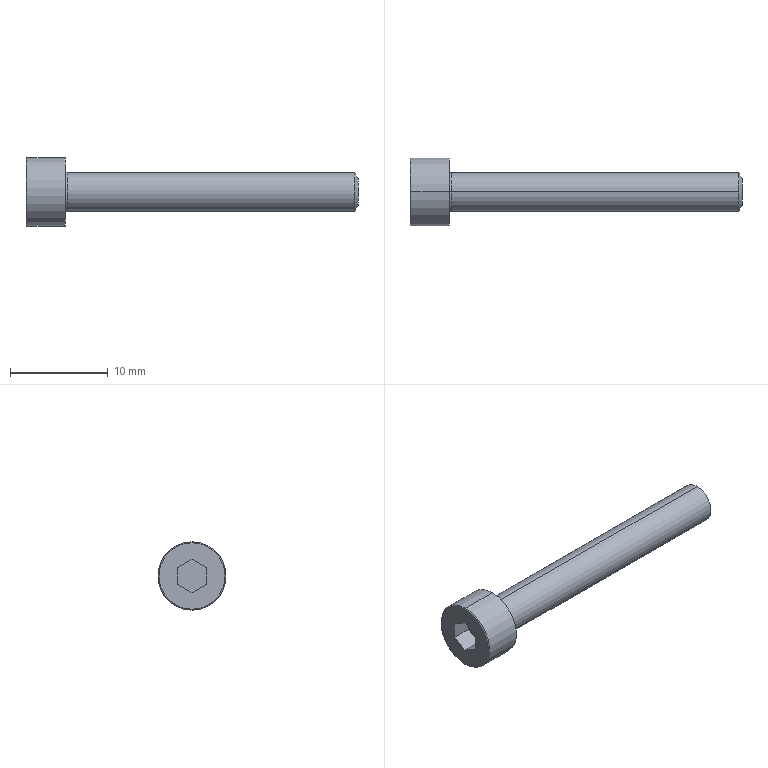Part | NX | features BREP 1 | 1 solid | 20 faces | box 34 x 7 x 7 mm | volume 514.422 mm3 | plane 10 | torus 4 | cylinder 4 | cone 2 | commonest cylinder face diameters 4 x2 7 x2
STEP:
#1=CARTESIAN_POINT('',(0.,0.,3.4));
#2=VERTEX_POINT('',#1);
#3=CARTESIAN_POINT('',(0.,0.,-3.4));
#4=VERTEX_POINT('',#3);
#5=CARTESIAN_POINT('',(0.,0.,0.));
#6=DIRECTION('',(-1.,0.,0.));
#7=DIRECTION('',(0.,0.,-1.));
#8=AXIS2_PLACEMENT_3D('',#5,#6,#7);
#9=CIRCLE('',#8,3.4);
#10=EDGE_CURVE('',#2,#4,#9,.T.);
#11=ORIENTED_EDGE('',*,*,#10,.F.);
#12=CARTESIAN_POINT('',(0.1,0.,3.5));
#13=VERTEX_POINT('',#12);
#14=CARTESIAN_POINT('',(0.1,0.,3.4));
#15=DIRECTION('',(0.,1.,0.));
#16=DIRECTION('',(0.,0.,1.));
#17=AXIS2_PLACEMENT_3D('',#14,#15,#16);
#18=CIRCLE('',#17,0.1);
#19=EDGE_CURVE('',#2,#13,#18,.T.);
#20=ORIENTED_EDGE('',*,*,#19,.T.);
#21=CARTESIAN_POINT('',(0.1,0.,-3.5));
#22=VERTEX_POINT('',#21);
#23=CARTESIAN_POINT('',(0.1,0.,0.));
#24=DIRECTION('',(1.,0.,0.));
#25=DIRECTION('',(0.,0.,-1.));
#26=AXIS2_PLACEMENT_3D('',#23,#24,#25);
#27=CIRCLE('',#26,3.5);
#28=EDGE_CURVE('',#22,#13,#27,.T.);
#29=ORIENTED_EDGE('',*,*,#28,.F.);
#30=CARTESIAN_POINT('',(0.1,0.,-3.4));
#31=DIRECTION('',(0.,-1.,0.));
#32=DIRECTION('',(0.,0.,-1.));
#33=AXIS2_PLACEMENT_3D('',#30,#31,#32);
#34=CIRCLE('',#33,0.1);
#35=EDGE_CURVE('',#4,#22,#34,.T.);
#36=ORIENTED_EDGE('',*,*,#35,.F.);
#37=EDGE_LOOP('',(#11,#20,#29,#36));
#38=FACE_BOUND('',#37,.T.);
#39=CARTESIAN_POINT('',(0.1,0.,0.));
#40=DIRECTION('',(1.,0.,0.));
#41=DIRECTION('',(0.,0.,-1.));
#42=AXIS2_PLACEMENT_3D('',#39,#40,#41);
#43=TOROIDAL_SURFACE('',#42,3.4,0.1);
#44=ADVANCED_FACE('',(#38),#43,.T.);
#45=CARTESIAN_POINT('',(34.,0.,1.394));
#46=VERTEX_POINT('',#45);
#47=CARTESIAN_POINT('',(34.,0.,-1.394));
#48=VERTEX_POINT('',#47);
#49=CARTESIAN_POINT('',(34.,0.,0.));
#50=DIRECTION('',(-1.,0.,0.));
#51=DIRECTION('',(0.,0.,1.));
#52=AXIS2_PLACEMENT_3D('',#49,#50,#51);
#53=CIRCLE('',#52,1.394);
#54=EDGE_CURVE('',#46,#48,#53,.T.);
#55=ORIENTED_EDGE('',*,*,#54,.T.);
#56=CARTESIAN_POINT('',(33.65,0.,-2.));
#57=VERTEX_POINT('',#56);
#58=CARTESIAN_POINT('',(33.65,0.,-2.));
#59=DIRECTION('',(-0.5,0.,-0.866));
#60=VECTOR('',#59,1000.);
#61=LINE('',#58,#60);
#62=EDGE_CURVE('',#57,#48,#61,.F.);
#63=ORIENTED_EDGE('',*,*,#62,.F.);
#64=CARTESIAN_POINT('',(33.65,0.,2.));
#65=VERTEX_POINT('',#64);
#66=CARTESIAN_POINT('',(33.65,0.,0.));
#67=DIRECTION('',(-1.,0.,0.));
#68=DIRECTION('',(0.,0.,1.));
#69=AXIS2_PLACEMENT_3D('',#66,#67,#68);
#70=CIRCLE('',#69,2.);
#71=EDGE_CURVE('',#65,#57,#70,.T.);
#72=ORIENTED_EDGE('',*,*,#71,.F.);
#73=CARTESIAN_POINT('',(33.65,0.,2.));
#74=DIRECTION('',(-0.5,0.,0.866));
#75=VECTOR('',#74,1000.);
#76=LINE('',#73,#75);
#77=EDGE_CURVE('',#65,#46,#76,.F.);
#78=ORIENTED_EDGE('',*,*,#77,.T.);
#79=EDGE_LOOP('',(#55,#63,#72,#78));
#80=FACE_BOUND('',#79,.T.);
#81=CARTESIAN_POINT('',(33.65,0.,0.));
#82=DIRECTION('',(-1.,0.,0.));
#83=DIRECTION('',(0.,0.,1.));
#84=AXIS2_PLACEMENT_3D('',#81,#82,#83);
#85=CONICAL_SURFACE('',#84,2.,1.047);
#86=ADVANCED_FACE('',(#80),#85,.T.);
#87=CARTESIAN_POINT('',(4.,0.,-2.2));
#88=VERTEX_POINT('',#87);
#89=CARTESIAN_POINT('',(4.,0.,2.2));
#90=VERTEX_POINT('',#89);
#91=CARTESIAN_POINT('',(4.,0.,0.));
#92=DIRECTION('',(-1.,0.,0.));
#93=DIRECTION('',(0.,0.,1.));
#94=AXIS2_PLACEMENT_3D('',#91,#92,#93);
#95=CIRCLE('',#94,2.2);
#96=EDGE_CURVE('',#88,#90,#95,.T.);
#97=ORIENTED_EDGE('',*,*,#96,.F.);
#98=CARTESIAN_POINT('',(4.2,0.,-2.));
#99=VERTEX_POINT('',#98);
#100=CARTESIAN_POINT('',(4.2,0.,-2.2));
#101=DIRECTION('',(0.,1.,0.));
#102=DIRECTION('',(0.,0.,1.));
#103=AXIS2_PLACEMENT_3D('',#100,#101,#102);
#104=CIRCLE('',#103,0.2);
#105=EDGE_CURVE('',#99,#88,#104,.F.);
#106=ORIENTED_EDGE('',*,*,#105,.F.);
#107=CARTESIAN_POINT('',(4.2,0.,2.));
#108=VERTEX_POINT('',#107);
#109=CARTESIAN_POINT('',(4.2,0.,0.));
#110=DIRECTION('',(-1.,0.,0.));
#111=DIRECTION('',(0.,0.,1.));
#112=AXIS2_PLACEMENT_3D('',#109,#110,#111);
#113=CIRCLE('',#112,2.);
#114=EDGE_CURVE('',#99,#108,#113,.T.);
#115=ORIENTED_EDGE('',*,*,#114,.T.);
#116=CARTESIAN_POINT('',(4.2,0.,2.2));
#117=DIRECTION('',(0.,-1.,0.));
#118=DIRECTION('',(0.,0.,-1.));
#119=AXIS2_PLACEMENT_3D('',#116,#117,#118);
#120=CIRCLE('',#119,0.2);
#121=EDGE_CURVE('',#108,#90,#120,.F.);
#122=ORIENTED_EDGE('',*,*,#121,.T.);
#123=EDGE_LOOP('',(#97,#106,#115,#122));
#124=FACE_BOUND('',#123,.T.);
#125=CARTESIAN_POINT('',(4.2,0.,0.));
#126=DIRECTION('',(-1.,0.,0.));
#127=DIRECTION('',(0.,0.,1.));
#128=AXIS2_PLACEMENT_3D('',#125,#126,#127);
#129=TOROIDAL_SURFACE('',#128,2.2,0.2);
#130=ADVANCED_FACE('',(#124),#129,.F.);
#131=CARTESIAN_POINT('',(4.,0.,3.5));
#132=VERTEX_POINT('',#131);
#133=CARTESIAN_POINT('',(4.,0.,-3.5));
#134=VERTEX_POINT('',#133);
#135=CARTESIAN_POINT('',(4.,0.,0.));
#136=DIRECTION('',(-1.,0.,0.));
#137=DIRECTION('',(0.,0.,1.));
#138=AXIS2_PLACEMENT_3D('',#135,#136,#137);
#139=CIRCLE('',#138,3.5);
#140=EDGE_CURVE('',#132,#134,#139,.T.);
#141=ORIENTED_EDGE('',*,*,#140,.T.);
#142=CARTESIAN_POINT('',(0.,0.,-3.5));
#143=DIRECTION('',(-1.,0.,0.));
#144=VECTOR('',#143,1000.);
#145=LINE('',#142,#144);
#146=EDGE_CURVE('',#22,#134,#145,.F.);
#147=ORIENTED_EDGE('',*,*,#146,.F.);
#148=ORIENTED_EDGE('',*,*,#28,.T.);
#149=CARTESIAN_POINT('',(0.,0.,3.5));
#150=DIRECTION('',(-1.,0.,0.));
#151=VECTOR('',#150,1000.);
#152=LINE('',#149,#151);
#153=EDGE_CURVE('',#13,#132,#152,.F.);
#154=ORIENTED_EDGE('',*,*,#153,.T.);
#155=EDGE_LOOP('',(#141,#147,#148,#154));
#156=FACE_BOUND('',#155,.T.);
#157=CARTESIAN_POINT('',(0.,0.,0.));
#158=DIRECTION('',(-1.,0.,0.));
#159=DIRECTION('',(0.,0.,1.));
#160=AXIS2_PLACEMENT_3D('',#157,#158,#159);
#161=CYLINDRICAL_SURFACE('',#160,3.5);
#162=ADVANCED_FACE('',(#156),#161,.T.);
#163=ORIENTED_EDGE('',*,*,#71,.T.);
#164=CARTESIAN_POINT('',(0.,0.,-2.));
#165=DIRECTION('',(-1.,0.,0.));
#166=VECTOR('',#165,1000.);
#167=LINE('',#164,#166);
#168=EDGE_CURVE('',#99,#57,#167,.F.);
#169=ORIENTED_EDGE('',*,*,#168,.F.);
#170=CARTESIAN_POINT('',(4.2,0.,0.));
#171=DIRECTION('',(-1.,0.,0.));
#172=DIRECTION('',(0.,0.,1.));
#173=AXIS2_PLACEMENT_3D('',#170,#171,#172);
#174=CIRCLE('',#173,2.);
#175=EDGE_CURVE('',#108,#99,#174,.T.);
#176=ORIENTED_EDGE('',*,*,#175,.F.);
#177=CARTESIAN_POINT('',(0.,0.,2.));
#178=DIRECTION('',(-1.,0.,0.));
#179=VECTOR('',#178,1000.);
#180=LINE('',#177,#179);
#181=EDGE_CURVE('',#108,#65,#180,.F.);
#182=ORIENTED_EDGE('',*,*,#181,.T.);
#183=EDGE_LOOP('',(#163,#169,#176,#182));
#184=FACE_BOUND('',#183,.T.);
#185=CARTESIAN_POINT('',(0.,0.,0.));
#186=DIRECTION('',(-1.,0.,0.));
#187=DIRECTION('',(0.,0.,1.));
#188=AXIS2_PLACEMENT_3D('',#185,#186,#187);
#189=CYLINDRICAL_SURFACE('',#188,2.);
#190=ADVANCED_FACE('',(#184),#189,.T.);
#191=ORIENTED_EDGE('',*,*,#168,.T.);
#192=CARTESIAN_POINT('',(33.65,0.,0.));
#193=DIRECTION('',(-1.,0.,0.));
#194=DIRECTION('',(0.,0.,1.));
#195=AXIS2_PLACEMENT_3D('',#192,#193,#194);
#196=CIRCLE('',#195,2.);
#197=EDGE_CURVE('',#57,#65,#196,.T.);
#198=ORIENTED_EDGE('',*,*,#197,.T.);
#199=ORIENTED_EDGE('',*,*,#181,.F.);
#200=ORIENTED_EDGE('',*,*,#114,.F.);
#201=EDGE_LOOP('',(#191,#198,#199,#200));
#202=FACE_BOUND('',#201,.T.);
#203=CARTESIAN_POINT('',(0.,0.,0.));
#204=DIRECTION('',(-1.,0.,0.));
#205=DIRECTION('',(0.,0.,1.));
#206=AXIS2_PLACEMENT_3D('',#203,#204,#205);
#207=CYLINDRICAL_SURFACE('',#206,2.);
#208=ADVANCED_FACE('',(#202),#207,.T.);
#209=CARTESIAN_POINT('',(0.,0.,0.));
#210=DIRECTION('',(-1.,0.,0.));
#211=DIRECTION('',(0.,0.,-1.));
#212=AXIS2_PLACEMENT_3D('',#209,#210,#211);
#213=CIRCLE('',#212,3.4);
#214=EDGE_CURVE('',#4,#2,#213,.T.);
#215=ORIENTED_EDGE('',*,*,#214,.T.);
#216=ORIENTED_EDGE('',*,*,#10,.T.);
#217=EDGE_LOOP('',(#215,#216));
#218=FACE_BOUND('',#217,.T.);
#219=CARTESIAN_POINT('',(0.,0.,1.72));
#220=VERTEX_POINT('',#219);
#221=CARTESIAN_POINT('',(0.,1.49,0.86));
#222=VERTEX_POINT('',#221);
#223=CARTESIAN_POINT('',(0.,0.,1.72));
#224=DIRECTION('',(0.,0.866,-0.5));
#225=VECTOR('',#224,1000.);
#226=LINE('',#223,#225);
#227=EDGE_CURVE('',#220,#222,#226,.T.);
#228=ORIENTED_EDGE('',*,*,#227,.F.);
#229=CARTESIAN_POINT('',(0.,-1.49,0.86));
#230=VERTEX_POINT('',#229);
#231=CARTESIAN_POINT('',(0.,-1.49,0.86));
#232=DIRECTION('',(0.,0.866,0.5));
#233=VECTOR('',#232,1000.);
#234=LINE('',#231,#233);
#235=EDGE_CURVE('',#230,#220,#234,.T.);
#236=ORIENTED_EDGE('',*,*,#235,.F.);
#237=CARTESIAN_POINT('',(0.,-1.49,-0.86));
#238=VERTEX_POINT('',#237);
#239=CARTESIAN_POINT('',(0.,-1.49,-0.86));
#240=DIRECTION('',(0.,0.,1.));
#241=VECTOR('',#240,1000.);
#242=LINE('',#239,#241);
#243=EDGE_CURVE('',#238,#230,#242,.T.);
#244=ORIENTED_EDGE('',*,*,#243,.F.);
#245=CARTESIAN_POINT('',(0.,0.,-1.72));
#246=VERTEX_POINT('',#245);
#247=CARTESIAN_POINT('',(0.,0.,-1.72));
#248=DIRECTION('',(0.,-0.866,0.5));
#249=VECTOR('',#248,1000.);
#250=LINE('',#247,#249);
#251=EDGE_CURVE('',#246,#238,#250,.T.);
#252=ORIENTED_EDGE('',*,*,#251,.F.);
#253=CARTESIAN_POINT('',(0.,1.49,-0.86));
#254=VERTEX_POINT('',#253);
#255=CARTESIAN_POINT('',(0.,1.49,-0.86));
#256=DIRECTION('',(0.,-0.866,-0.5));
#257=VECTOR('',#256,1000.);
#258=LINE('',#255,#257);
#259=EDGE_CURVE('',#254,#246,#258,.T.);
#260=ORIENTED_EDGE('',*,*,#259,.F.);
#261=CARTESIAN_POINT('',(0.,1.49,0.86));
#262=DIRECTION('',(0.,0.,-1.));
#263=VECTOR('',#262,1000.);
#264=LINE('',#261,#263);
#265=EDGE_CURVE('',#222,#254,#264,.T.);
#266=ORIENTED_EDGE('',*,*,#265,.F.);
#267=EDGE_LOOP('',(#228,#236,#244,#252,#260,#266));
#268=FACE_BOUND('',#267,.T.);
#269=CARTESIAN_POINT('',(0.,0.,0.));
#270=DIRECTION('',(1.,0.,0.));
#271=DIRECTION('',(0.,1.,0.));
#272=AXIS2_PLACEMENT_3D('',#269,#270,#271);
#273=PLANE('',#272);
#274=ADVANCED_FACE('',(#218,#268),#273,.F.);
#275=ORIENTED_EDGE('',*,*,#146,.T.);
#276=CARTESIAN_POINT('',(4.,0.,0.));
#277=DIRECTION('',(-1.,0.,0.));
#278=DIRECTION('',(0.,0.,1.));
#279=AXIS2_PLACEMENT_3D('',#276,#277,#278);
#280=CIRCLE('',#279,3.5);
#281=EDGE_CURVE('',#134,#132,#280,.T.);
#282=ORIENTED_EDGE('',*,*,#281,.T.);
#283=ORIENTED_EDGE('',*,*,#153,.F.);
#284=CARTESIAN_POINT('',(0.1,0.,0.));
#285=DIRECTION('',(1.,0.,0.));
#286=DIRECTION('',(0.,0.,-1.));
#287=AXIS2_PLACEMENT_3D('',#284,#285,#286);
#288=CIRCLE('',#287,3.5);
#289=EDGE_CURVE('',#13,#22,#288,.T.);
#290=ORIENTED_EDGE('',*,*,#289,.T.);
#291=EDGE_LOOP('',(#275,#282,#283,#290));
#292=FACE_BOUND('',#291,.T.);
#293=CARTESIAN_POINT('',(0.,0.,0.));
#294=DIRECTION('',(-1.,0.,0.));
#295=DIRECTION('',(0.,0.,1.));
#296=AXIS2_PLACEMENT_3D('',#293,#294,#295);
#297=CYLINDRICAL_SURFACE('',#296,3.5);
#298=ADVANCED_FACE('',(#292),#297,.T.);
#299=ORIENTED_EDGE('',*,*,#140,.F.);
#300=ORIENTED_EDGE('',*,*,#281,.F.);
#301=EDGE_LOOP('',(#299,#300));
#302=FACE_BOUND('',#301,.T.);
#303=CARTESIAN_POINT('',(4.,0.,0.));
#304=DIRECTION('',(-1.,0.,0.));
#305=DIRECTION('',(0.,0.,1.));
#306=AXIS2_PLACEMENT_3D('',#303,#304,#305);
#307=CIRCLE('',#306,2.2);
#308=EDGE_CURVE('',#90,#88,#307,.T.);
#309=ORIENTED_EDGE('',*,*,#308,.T.);
#310=ORIENTED_EDGE('',*,*,#96,.T.);
#311=EDGE_LOOP('',(#309,#310));
#312=FACE_BOUND('',#311,.T.);
#313=CARTESIAN_POINT('',(4.,3.5,0.));
#314=DIRECTION('',(-1.,0.,0.));
#315=DIRECTION('',(0.,0.,1.));
#316=AXIS2_PLACEMENT_3D('',#313,#314,#315);
#317=PLANE('',#316);
#318=ADVANCED_FACE('',(#302,#312),#317,.F.);
#319=ORIENTED_EDGE('',*,*,#105,.T.);
#320=ORIENTED_EDGE('',*,*,#308,.F.);
#321=ORIENTED_EDGE('',*,*,#121,.F.);
#322=ORIENTED_EDGE('',*,*,#175,.T.);
#323=EDGE_LOOP('',(#319,#320,#321,#322));
#324=FACE_BOUND('',#323,.T.);
#325=CARTESIAN_POINT('',(4.2,0.,0.));
#326=DIRECTION('',(-1.,0.,0.));
#327=DIRECTION('',(0.,0.,1.));
#328=AXIS2_PLACEMENT_3D('',#325,#326,#327);
#329=TOROIDAL_SURFACE('',#328,2.2,0.2);
#330=ADVANCED_FACE('',(#324),#329,.F.);
#331=ORIENTED_EDGE('',*,*,#235,.T.);
#332=CARTESIAN_POINT('',(2.,0.,1.72));
#333=VERTEX_POINT('',#332);
#334=CARTESIAN_POINT('',(2.,0.,1.72));
#335=DIRECTION('',(-1.,0.,0.));
#336=VECTOR('',#335,1000.);
#337=LINE('',#334,#336);
#338=EDGE_CURVE('',#333,#220,#337,.T.);
#339=ORIENTED_EDGE('',*,*,#338,.F.);
#340=CARTESIAN_POINT('',(2.,-1.49,0.86));
#341=VERTEX_POINT('',#340);
#342=CARTESIAN_POINT('',(2.,-1.49,0.86));
#343=DIRECTION('',(0.,0.866,0.5));
#344=VECTOR('',#343,1000.);
#345=LINE('',#342,#344);
#346=EDGE_CURVE('',#341,#333,#345,.T.);
#347=ORIENTED_EDGE('',*,*,#346,.F.);
#348=CARTESIAN_POINT('',(2.,-1.49,0.86));
#349=DIRECTION('',(-1.,0.,0.));
#350=VECTOR('',#349,1000.);
#351=LINE('',#348,#350);
#352=EDGE_CURVE('',#341,#230,#351,.T.);
#353=ORIENTED_EDGE('',*,*,#352,.T.);
#354=EDGE_LOOP('',(#331,#339,#347,#353));
#355=FACE_BOUND('',#354,.T.);
#356=CARTESIAN_POINT('',(2.,-1.49,0.86));
#357=DIRECTION('',(0.,-0.5,0.866));
#358=DIRECTION('',(-1.,0.,0.));
#359=AXIS2_PLACEMENT_3D('',#356,#357,#358);
#360=PLANE('',#359);
#361=ADVANCED_FACE('',(#355),#360,.F.);
#362=ORIENTED_EDGE('',*,*,#243,.T.);
#363=ORIENTED_EDGE('',*,*,#352,.F.);
#364=CARTESIAN_POINT('',(2.,-1.49,-0.86));
#365=VERTEX_POINT('',#364);
#366=CARTESIAN_POINT('',(2.,-1.49,-0.86));
#367=DIRECTION('',(0.,0.,1.));
#368=VECTOR('',#367,1000.);
#369=LINE('',#366,#368);
#370=EDGE_CURVE('',#365,#341,#369,.T.);
#371=ORIENTED_EDGE('',*,*,#370,.F.);
#372=CARTESIAN_POINT('',(2.,-1.49,-0.86));
#373=DIRECTION('',(-1.,0.,0.));
#374=VECTOR('',#373,1000.);
#375=LINE('',#372,#374);
#376=EDGE_CURVE('',#365,#238,#375,.T.);
#377=ORIENTED_EDGE('',*,*,#376,.T.);
#378=EDGE_LOOP('',(#362,#363,#371,#377));
#379=FACE_BOUND('',#378,.T.);
#380=CARTESIAN_POINT('',(2.,-1.49,-0.86));
#381=DIRECTION('',(0.,-1.,0.));
#382=DIRECTION('',(0.,0.,-1.));
#383=AXIS2_PLACEMENT_3D('',#380,#381,#382);
#384=PLANE('',#383);
#385=ADVANCED_FACE('',(#379),#384,.F.);
#386=ORIENTED_EDGE('',*,*,#251,.T.);
#387=ORIENTED_EDGE('',*,*,#376,.F.);
#388=CARTESIAN_POINT('',(2.,0.,-1.72));
#389=VERTEX_POINT('',#388);
#390=CARTESIAN_POINT('',(2.,0.,-1.72));
#391=DIRECTION('',(0.,-0.866,0.5));
#392=VECTOR('',#391,1000.);
#393=LINE('',#390,#392);
#394=EDGE_CURVE('',#389,#365,#393,.T.);
#395=ORIENTED_EDGE('',*,*,#394,.F.);
#396=CARTESIAN_POINT('',(2.,0.,-1.72));
#397=DIRECTION('',(-1.,0.,0.));
#398=VECTOR('',#397,1000.);
#399=LINE('',#396,#398);
#400=EDGE_CURVE('',#389,#246,#399,.T.);
#401=ORIENTED_EDGE('',*,*,#400,.T.);
#402=EDGE_LOOP('',(#386,#387,#395,#401));
#403=FACE_BOUND('',#402,.T.);
#404=CARTESIAN_POINT('',(2.,0.,-1.72));
#405=DIRECTION('',(0.,-0.5,-0.866));
#406=DIRECTION('',(0.,-0.866,0.5));
#407=AXIS2_PLACEMENT_3D('',#404,#405,#406);
#408=PLANE('',#407);
#409=ADVANCED_FACE('',(#403),#408,.F.);
#410=ORIENTED_EDGE('',*,*,#259,.T.);
#411=ORIENTED_EDGE('',*,*,#400,.F.);
#412=CARTESIAN_POINT('',(2.,1.49,-0.86));
#413=VERTEX_POINT('',#412);
#414=CARTESIAN_POINT('',(2.,1.49,-0.86));
#415=DIRECTION('',(0.,-0.866,-0.5));
#416=VECTOR('',#415,1000.);
#417=LINE('',#414,#416);
#418=EDGE_CURVE('',#413,#389,#417,.T.);
#419=ORIENTED_EDGE('',*,*,#418,.F.);
#420=CARTESIAN_POINT('',(2.,1.49,-0.86));
#421=DIRECTION('',(-1.,0.,0.));
#422=VECTOR('',#421,1000.);
#423=LINE('',#420,#422);
#424=EDGE_CURVE('',#413,#254,#423,.T.);
#425=ORIENTED_EDGE('',*,*,#424,.T.);
#426=EDGE_LOOP('',(#410,#411,#419,#425));
#427=FACE_BOUND('',#426,.T.);
#428=CARTESIAN_POINT('',(2.,1.49,-0.86));
#429=DIRECTION('',(0.,0.5,-0.866));
#430=DIRECTION('',(-1.,0.,0.));
#431=AXIS2_PLACEMENT_3D('',#428,#429,#430);
#432=PLANE('',#431);
#433=ADVANCED_FACE('',(#427),#432,.F.);
#434=ORIENTED_EDGE('',*,*,#265,.T.);
#435=ORIENTED_EDGE('',*,*,#424,.F.);
#436=CARTESIAN_POINT('',(2.,1.49,0.86));
#437=VERTEX_POINT('',#436);
#438=CARTESIAN_POINT('',(2.,1.49,0.86));
#439=DIRECTION('',(0.,0.,-1.));
#440=VECTOR('',#439,1000.);
#441=LINE('',#438,#440);
#442=EDGE_CURVE('',#437,#413,#441,.T.);
#443=ORIENTED_EDGE('',*,*,#442,.F.);
#444=CARTESIAN_POINT('',(2.,1.49,0.86));
#445=DIRECTION('',(-1.,0.,0.));
#446=VECTOR('',#445,1000.);
#447=LINE('',#444,#446);
#448=EDGE_CURVE('',#437,#222,#447,.T.);
#449=ORIENTED_EDGE('',*,*,#448,.T.);
#450=EDGE_LOOP('',(#434,#435,#443,#449));
#451=FACE_BOUND('',#450,.T.);
#452=CARTESIAN_POINT('',(2.,1.49,0.86));
#453=DIRECTION('',(0.,1.,0.));
#454=DIRECTION('',(1.,0.,0.));
#455=AXIS2_PLACEMENT_3D('',#452,#453,#454);
#456=PLANE('',#455);
#457=ADVANCED_FACE('',(#451),#456,.F.);
#458=ORIENTED_EDGE('',*,*,#227,.T.);
#459=ORIENTED_EDGE('',*,*,#448,.F.);
#460=CARTESIAN_POINT('',(2.,0.,1.72));
#461=DIRECTION('',(0.,0.866,-0.5));
#462=VECTOR('',#461,1000.);
#463=LINE('',#460,#462);
#464=EDGE_CURVE('',#333,#437,#463,.T.);
#465=ORIENTED_EDGE('',*,*,#464,.F.);
#466=ORIENTED_EDGE('',*,*,#338,.T.);
#467=EDGE_LOOP('',(#458,#459,#465,#466));
#468=FACE_BOUND('',#467,.T.);
#469=CARTESIAN_POINT('',(2.,0.,1.72));
#470=DIRECTION('',(0.,0.5,0.866));
#471=DIRECTION('',(1.,0.,0.));
#472=AXIS2_PLACEMENT_3D('',#469,#470,#471);
#473=PLANE('',#472);
#474=ADVANCED_FACE('',(#468),#473,.F.);
#475=ORIENTED_EDGE('',*,*,#346,.T.);
#476=ORIENTED_EDGE('',*,*,#464,.T.);
#477=ORIENTED_EDGE('',*,*,#442,.T.);
#478=ORIENTED_EDGE('',*,*,#418,.T.);
#479=ORIENTED_EDGE('',*,*,#394,.T.);
#480=ORIENTED_EDGE('',*,*,#370,.T.);
#481=EDGE_LOOP('',(#475,#476,#477,#478,#479,#480));
#482=FACE_BOUND('',#481,.T.);
#483=CARTESIAN_POINT('',(2.,1.49,2.58));
#484=DIRECTION('',(-1.,0.,0.));
#485=DIRECTION('',(0.,0.,1.));
#486=AXIS2_PLACEMENT_3D('',#483,#484,#485);
#487=PLANE('',#486);
#488=ADVANCED_FACE('',(#482),#487,.T.);
#489=ORIENTED_EDGE('',*,*,#62,.T.);
#490=CARTESIAN_POINT('',(34.,0.,0.));
#491=DIRECTION('',(-1.,0.,0.));
#492=DIRECTION('',(0.,0.,1.));
#493=AXIS2_PLACEMENT_3D('',#490,#491,#492);
#494=CIRCLE('',#493,1.394);
#495=EDGE_CURVE('',#48,#46,#494,.T.);
#496=ORIENTED_EDGE('',*,*,#495,.T.);
#497=ORIENTED_EDGE('',*,*,#77,.F.);
#498=ORIENTED_EDGE('',*,*,#197,.F.);
#499=EDGE_LOOP('',(#489,#496,#497,#498));
#500=FACE_BOUND('',#499,.T.);
#501=CARTESIAN_POINT('',(33.65,0.,0.));
#502=DIRECTION('',(-1.,0.,0.));
#503=DIRECTION('',(0.,0.,1.));
#504=AXIS2_PLACEMENT_3D('',#501,#502,#503);
#505=CONICAL_SURFACE('',#504,2.,1.047);
#506=ADVANCED_FACE('',(#500),#505,.T.);
#507=ORIENTED_EDGE('',*,*,#54,.F.);
#508=ORIENTED_EDGE('',*,*,#495,.F.);
#509=EDGE_LOOP('',(#507,#508));
#510=FACE_BOUND('',#509,.T.);
#511=CARTESIAN_POINT('',(34.,2.,0.));
#512=DIRECTION('',(-1.,0.,0.));
#513=DIRECTION('',(0.,0.,1.));
#514=AXIS2_PLACEMENT_3D('',#511,#512,#513);
#515=PLANE('',#514);
#516=ADVANCED_FACE('',(#510),#515,.F.);
#517=ORIENTED_EDGE('',*,*,#19,.F.);
#518=ORIENTED_EDGE('',*,*,#214,.F.);
#519=ORIENTED_EDGE('',*,*,#35,.T.);
#520=ORIENTED_EDGE('',*,*,#289,.F.);
#521=EDGE_LOOP('',(#517,#518,#519,#520));
#522=FACE_BOUND('',#521,.T.);
#523=CARTESIAN_POINT('',(0.1,0.,0.));
#524=DIRECTION('',(1.,0.,0.));
#525=DIRECTION('',(0.,0.,-1.));
#526=AXIS2_PLACEMENT_3D('',#523,#524,#525);
#527=TOROIDAL_SURFACE('',#526,3.4,0.1);
#528=ADVANCED_FACE('',(#522),#527,.T.);
#529=CLOSED_SHELL('',(#44,#86,#130,#162,#190,#208,#274,#298,#318,#330,#361,#385,#409,#433,#457,#474,#488,#506,#516,#528));
#530=MANIFOLD_SOLID_BREP('',#529);
#531=(LENGTH_UNIT()NAMED_UNIT(*)SI_UNIT(.MILLI.,.METRE.));
#532=UNCERTAINTY_MEASURE_WITH_UNIT(LENGTH_MEASURE(0.00001),#531,'','');
#533=(NAMED_UNIT(*)PLANE_ANGLE_UNIT()SI_UNIT($,.RADIAN.));
#534=(NAMED_UNIT(*)SI_UNIT($,.STERADIAN.)SOLID_ANGLE_UNIT());
#535=(GEOMETRIC_REPRESENTATION_CONTEXT(3)GLOBAL_UNCERTAINTY_ASSIGNED_CONTEXT((#532))GLOBAL_UNIT_ASSIGNED_CONTEXT((#531,#533,#534))REPRESENTATION_CONTEXT('',''));
#536=ADVANCED_BREP_SHAPE_REPRESENTATION('',(#530),#535);